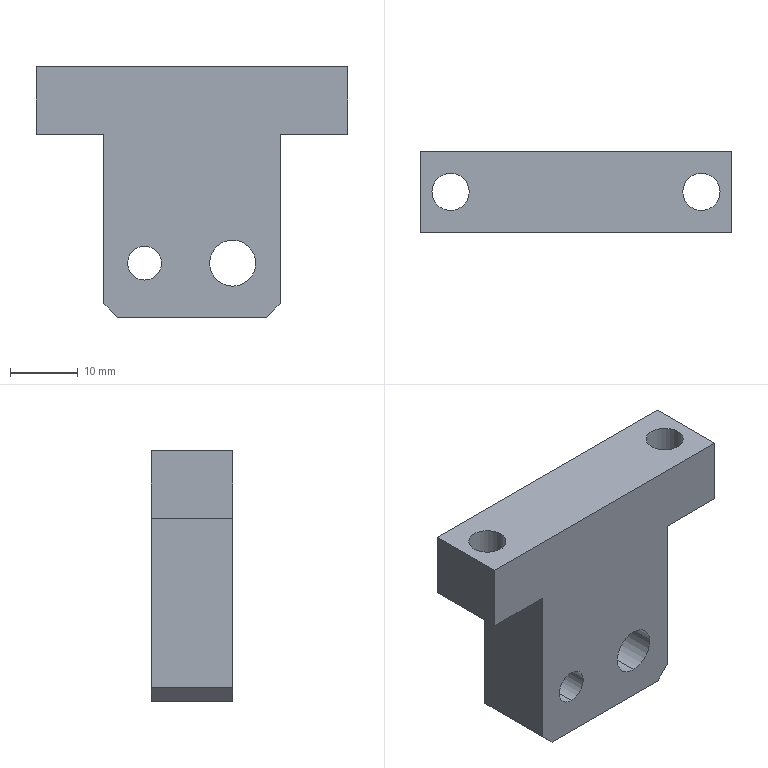Part | NX | features BREP 1 | 1 solid | 20 faces | box 46 x 12 x 37 mm | volume 12749 mm3 | plane 12 | cylinder 8 | commonest cylinder face diameters 5.5 x4 5 x2 6.8 x2
STEP:
#1=CARTESIAN_POINT('',(-20.051,-130.878,4.6));
#2=VERTEX_POINT('',#1);
#3=CARTESIAN_POINT('',(-20.051,-130.878,11.4));
#4=VERTEX_POINT('',#3);
#5=CARTESIAN_POINT('',(-20.051,-130.878,8.));
#6=DIRECTION('',(0.,1.,0.));
#7=DIRECTION('',(0.,0.,1.));
#8=AXIS2_PLACEMENT_3D('',#5,#6,#7);
#9=CIRCLE('',#8,3.4);
#10=EDGE_CURVE('',#2,#4,#9,.T.);
#11=ORIENTED_EDGE('',*,*,#10,.F.);
#12=CARTESIAN_POINT('',(-20.051,-118.878,4.6));
#13=VERTEX_POINT('',#12);
#14=CARTESIAN_POINT('',(-20.051,-118.878,4.6));
#15=DIRECTION('',(0.,1.,0.));
#16=VECTOR('',#15,1000.);
#17=LINE('',#14,#16);
#18=EDGE_CURVE('',#13,#2,#17,.F.);
#19=ORIENTED_EDGE('',*,*,#18,.F.);
#20=CARTESIAN_POINT('',(-20.051,-118.878,11.4));
#21=VERTEX_POINT('',#20);
#22=CARTESIAN_POINT('',(-20.051,-118.878,8.));
#23=DIRECTION('',(0.,1.,0.));
#24=DIRECTION('',(0.,0.,1.));
#25=AXIS2_PLACEMENT_3D('',#22,#23,#24);
#26=CIRCLE('',#25,3.4);
#27=EDGE_CURVE('',#13,#21,#26,.T.);
#28=ORIENTED_EDGE('',*,*,#27,.T.);
#29=CARTESIAN_POINT('',(-20.051,-118.878,11.4));
#30=DIRECTION('',(0.,1.,0.));
#31=VECTOR('',#30,1000.);
#32=LINE('',#29,#31);
#33=EDGE_CURVE('',#21,#4,#32,.F.);
#34=ORIENTED_EDGE('',*,*,#33,.T.);
#35=EDGE_LOOP('',(#11,#19,#28,#34));
#36=FACE_BOUND('',#35,.T.);
#37=CARTESIAN_POINT('',(-20.051,-118.878,8.));
#38=DIRECTION('',(0.,1.,0.));
#39=DIRECTION('',(0.,0.,1.));
#40=AXIS2_PLACEMENT_3D('',#37,#38,#39);
#41=CYLINDRICAL_SURFACE('',#40,3.4);
#42=ADVANCED_FACE('',(#36),#41,.F.);
#43=CARTESIAN_POINT('',(-41.801,-124.878,37.));
#44=VERTEX_POINT('',#43);
#45=CARTESIAN_POINT('',(-47.301,-124.878,37.));
#46=VERTEX_POINT('',#45);
#47=CARTESIAN_POINT('',(-44.551,-124.878,37.));
#48=DIRECTION('',(0.,0.,-1.));
#49=DIRECTION('',(-1.,0.,0.));
#50=AXIS2_PLACEMENT_3D('',#47,#48,#49);
#51=CIRCLE('',#50,2.75);
#52=EDGE_CURVE('',#44,#46,#51,.T.);
#53=ORIENTED_EDGE('',*,*,#52,.F.);
#54=CARTESIAN_POINT('',(-41.801,-124.878,27.));
#55=VERTEX_POINT('',#54);
#56=CARTESIAN_POINT('',(-41.801,-124.878,37.));
#57=DIRECTION('',(0.,0.,-1.));
#58=VECTOR('',#57,1000.);
#59=LINE('',#56,#58);
#60=EDGE_CURVE('',#44,#55,#59,.T.);
#61=ORIENTED_EDGE('',*,*,#60,.T.);
#62=CARTESIAN_POINT('',(-47.301,-124.878,27.));
#63=VERTEX_POINT('',#62);
#64=CARTESIAN_POINT('',(-44.551,-124.878,27.));
#65=DIRECTION('',(0.,0.,-1.));
#66=DIRECTION('',(-1.,0.,0.));
#67=AXIS2_PLACEMENT_3D('',#64,#65,#66);
#68=CIRCLE('',#67,2.75);
#69=EDGE_CURVE('',#55,#63,#68,.T.);
#70=ORIENTED_EDGE('',*,*,#69,.T.);
#71=CARTESIAN_POINT('',(-47.301,-124.878,37.));
#72=DIRECTION('',(0.,0.,-1.));
#73=VECTOR('',#72,1000.);
#74=LINE('',#71,#73);
#75=EDGE_CURVE('',#46,#63,#74,.T.);
#76=ORIENTED_EDGE('',*,*,#75,.F.);
#77=EDGE_LOOP('',(#53,#61,#70,#76));
#78=FACE_BOUND('',#77,.T.);
#79=CARTESIAN_POINT('',(-44.551,-124.878,37.));
#80=DIRECTION('',(0.,0.,-1.));
#81=DIRECTION('',(-1.,0.,0.));
#82=AXIS2_PLACEMENT_3D('',#79,#80,#81);
#83=CYLINDRICAL_SURFACE('',#82,2.75);
#84=ADVANCED_FACE('',(#78),#83,.F.);
#85=CARTESIAN_POINT('',(-4.801,-124.878,37.));
#86=VERTEX_POINT('',#85);
#87=CARTESIAN_POINT('',(-10.301,-124.878,37.));
#88=VERTEX_POINT('',#87);
#89=CARTESIAN_POINT('',(-7.551,-124.878,37.));
#90=DIRECTION('',(0.,0.,-1.));
#91=DIRECTION('',(-1.,0.,0.));
#92=AXIS2_PLACEMENT_3D('',#89,#90,#91);
#93=CIRCLE('',#92,2.75);
#94=EDGE_CURVE('',#86,#88,#93,.T.);
#95=ORIENTED_EDGE('',*,*,#94,.F.);
#96=CARTESIAN_POINT('',(-4.801,-124.878,27.));
#97=VERTEX_POINT('',#96);
#98=CARTESIAN_POINT('',(-4.801,-124.878,37.));
#99=DIRECTION('',(0.,0.,-1.));
#100=VECTOR('',#99,1000.);
#101=LINE('',#98,#100);
#102=EDGE_CURVE('',#86,#97,#101,.T.);
#103=ORIENTED_EDGE('',*,*,#102,.T.);
#104=CARTESIAN_POINT('',(-10.301,-124.878,27.));
#105=VERTEX_POINT('',#104);
#106=CARTESIAN_POINT('',(-7.551,-124.878,27.));
#107=DIRECTION('',(0.,0.,-1.));
#108=DIRECTION('',(-1.,0.,0.));
#109=AXIS2_PLACEMENT_3D('',#106,#107,#108);
#110=CIRCLE('',#109,2.75);
#111=EDGE_CURVE('',#97,#105,#110,.T.);
#112=ORIENTED_EDGE('',*,*,#111,.T.);
#113=CARTESIAN_POINT('',(-10.301,-124.878,37.));
#114=DIRECTION('',(0.,0.,-1.));
#115=VECTOR('',#114,1000.);
#116=LINE('',#113,#115);
#117=EDGE_CURVE('',#88,#105,#116,.T.);
#118=ORIENTED_EDGE('',*,*,#117,.F.);
#119=EDGE_LOOP('',(#95,#103,#112,#118));
#120=FACE_BOUND('',#119,.T.);
#121=CARTESIAN_POINT('',(-7.551,-124.878,37.));
#122=DIRECTION('',(0.,0.,-1.));
#123=DIRECTION('',(-1.,0.,0.));
#124=AXIS2_PLACEMENT_3D('',#121,#122,#123);
#125=CYLINDRICAL_SURFACE('',#124,2.75);
#126=ADVANCED_FACE('',(#120),#125,.F.);
#127=CARTESIAN_POINT('',(-33.051,-130.878,5.5));
#128=VERTEX_POINT('',#127);
#129=CARTESIAN_POINT('',(-33.051,-130.878,10.5));
#130=VERTEX_POINT('',#129);
#131=CARTESIAN_POINT('',(-33.051,-130.878,8.));
#132=DIRECTION('',(0.,1.,0.));
#133=DIRECTION('',(0.,0.,1.));
#134=AXIS2_PLACEMENT_3D('',#131,#132,#133);
#135=CIRCLE('',#134,2.5);
#136=EDGE_CURVE('',#128,#130,#135,.T.);
#137=ORIENTED_EDGE('',*,*,#136,.F.);
#138=CARTESIAN_POINT('',(-33.051,-118.878,5.5));
#139=VERTEX_POINT('',#138);
#140=CARTESIAN_POINT('',(-33.051,-118.878,5.5));
#141=DIRECTION('',(0.,1.,0.));
#142=VECTOR('',#141,1000.);
#143=LINE('',#140,#142);
#144=EDGE_CURVE('',#139,#128,#143,.F.);
#145=ORIENTED_EDGE('',*,*,#144,.F.);
#146=CARTESIAN_POINT('',(-33.051,-118.878,10.5));
#147=VERTEX_POINT('',#146);
#148=CARTESIAN_POINT('',(-33.051,-118.878,8.));
#149=DIRECTION('',(0.,1.,0.));
#150=DIRECTION('',(0.,0.,1.));
#151=AXIS2_PLACEMENT_3D('',#148,#149,#150);
#152=CIRCLE('',#151,2.5);
#153=EDGE_CURVE('',#139,#147,#152,.T.);
#154=ORIENTED_EDGE('',*,*,#153,.T.);
#155=CARTESIAN_POINT('',(-33.051,-118.878,10.5));
#156=DIRECTION('',(0.,1.,0.));
#157=VECTOR('',#156,1000.);
#158=LINE('',#155,#157);
#159=EDGE_CURVE('',#147,#130,#158,.F.);
#160=ORIENTED_EDGE('',*,*,#159,.T.);
#161=EDGE_LOOP('',(#137,#145,#154,#160));
#162=FACE_BOUND('',#161,.T.);
#163=CARTESIAN_POINT('',(-33.051,-118.878,8.));
#164=DIRECTION('',(0.,1.,0.));
#165=DIRECTION('',(0.,0.,1.));
#166=AXIS2_PLACEMENT_3D('',#163,#164,#165);
#167=CYLINDRICAL_SURFACE('',#166,2.5);
#168=ADVANCED_FACE('',(#162),#167,.F.);
#169=CARTESIAN_POINT('',(-13.051,-118.878,27.));
#170=VERTEX_POINT('',#169);
#171=CARTESIAN_POINT('',(-13.051,-118.878,2.));
#172=VERTEX_POINT('',#171);
#173=CARTESIAN_POINT('',(-13.051,-118.878,27.));
#174=DIRECTION('',(0.,0.,-1.));
#175=VECTOR('',#174,1000.);
#176=LINE('',#173,#175);
#177=EDGE_CURVE('',#170,#172,#176,.T.);
#178=ORIENTED_EDGE('',*,*,#177,.T.);
#179=CARTESIAN_POINT('',(-15.051,-118.878,0.));
#180=VERTEX_POINT('',#179);
#181=CARTESIAN_POINT('',(-13.051,-118.878,2.));
#182=DIRECTION('',(-0.7071,0.,-0.7071));
#183=VECTOR('',#182,1000.);
#184=LINE('',#181,#183);
#185=EDGE_CURVE('',#172,#180,#184,.T.);
#186=ORIENTED_EDGE('',*,*,#185,.T.);
#187=CARTESIAN_POINT('',(-37.051,-118.878,0.));
#188=VERTEX_POINT('',#187);
#189=CARTESIAN_POINT('',(-39.051,-118.878,0.));
#190=DIRECTION('',(-1.,0.,0.));
#191=VECTOR('',#190,1000.);
#192=LINE('',#189,#191);
#193=EDGE_CURVE('',#180,#188,#192,.T.);
#194=ORIENTED_EDGE('',*,*,#193,.T.);
#195=CARTESIAN_POINT('',(-39.051,-118.878,2.));
#196=VERTEX_POINT('',#195);
#197=CARTESIAN_POINT('',(-39.051,-118.878,2.));
#198=DIRECTION('',(-0.7071,0.,0.7071));
#199=VECTOR('',#198,1000.);
#200=LINE('',#197,#199);
#201=EDGE_CURVE('',#188,#196,#200,.T.);
#202=ORIENTED_EDGE('',*,*,#201,.T.);
#203=CARTESIAN_POINT('',(-39.051,-118.878,27.));
#204=VERTEX_POINT('',#203);
#205=CARTESIAN_POINT('',(-39.051,-118.878,27.));
#206=DIRECTION('',(0.,0.,-1.));
#207=VECTOR('',#206,1000.);
#208=LINE('',#205,#207);
#209=EDGE_CURVE('',#204,#196,#208,.T.);
#210=ORIENTED_EDGE('',*,*,#209,.F.);
#211=CARTESIAN_POINT('',(-49.051,-118.878,27.));
#212=VERTEX_POINT('',#211);
#213=CARTESIAN_POINT('',(-49.051,-118.878,27.));
#214=DIRECTION('',(-1.,0.,0.));
#215=VECTOR('',#214,1000.);
#216=LINE('',#213,#215);
#217=EDGE_CURVE('',#204,#212,#216,.T.);
#218=ORIENTED_EDGE('',*,*,#217,.T.);
#219=CARTESIAN_POINT('',(-49.051,-118.878,37.));
#220=VERTEX_POINT('',#219);
#221=CARTESIAN_POINT('',(-49.051,-118.878,37.));
#222=DIRECTION('',(0.,0.,-1.));
#223=VECTOR('',#222,1000.);
#224=LINE('',#221,#223);
#225=EDGE_CURVE('',#220,#212,#224,.T.);
#226=ORIENTED_EDGE('',*,*,#225,.F.);
#227=CARTESIAN_POINT('',(-3.051,-118.878,37.));
#228=VERTEX_POINT('',#227);
#229=CARTESIAN_POINT('',(-49.051,-118.878,37.));
#230=DIRECTION('',(-1.,0.,0.));
#231=VECTOR('',#230,1000.);
#232=LINE('',#229,#231);
#233=EDGE_CURVE('',#228,#220,#232,.T.);
#234=ORIENTED_EDGE('',*,*,#233,.F.);
#235=CARTESIAN_POINT('',(-3.051,-118.878,27.));
#236=VERTEX_POINT('',#235);
#237=CARTESIAN_POINT('',(-3.051,-118.878,37.));
#238=DIRECTION('',(0.,0.,-1.));
#239=VECTOR('',#238,1000.);
#240=LINE('',#237,#239);
#241=EDGE_CURVE('',#228,#236,#240,.T.);
#242=ORIENTED_EDGE('',*,*,#241,.T.);
#243=CARTESIAN_POINT('',(-49.051,-118.878,27.));
#244=DIRECTION('',(-1.,0.,0.));
#245=VECTOR('',#244,1000.);
#246=LINE('',#243,#245);
#247=EDGE_CURVE('',#236,#170,#246,.T.);
#248=ORIENTED_EDGE('',*,*,#247,.T.);
#249=EDGE_LOOP('',(#178,#186,#194,#202,#210,#218,#226,#234,#242,#248));
#250=FACE_BOUND('',#249,.T.);
#251=CARTESIAN_POINT('',(-33.051,-118.878,8.));
#252=DIRECTION('',(0.,1.,0.));
#253=DIRECTION('',(0.,0.,1.));
#254=AXIS2_PLACEMENT_3D('',#251,#252,#253);
#255=CIRCLE('',#254,2.5);
#256=EDGE_CURVE('',#147,#139,#255,.T.);
#257=ORIENTED_EDGE('',*,*,#256,.F.);
#258=ORIENTED_EDGE('',*,*,#153,.F.);
#259=EDGE_LOOP('',(#257,#258));
#260=FACE_BOUND('',#259,.T.);
#261=CARTESIAN_POINT('',(-20.051,-118.878,8.));
#262=DIRECTION('',(0.,1.,0.));
#263=DIRECTION('',(0.,0.,1.));
#264=AXIS2_PLACEMENT_3D('',#261,#262,#263);
#265=CIRCLE('',#264,3.4);
#266=EDGE_CURVE('',#21,#13,#265,.T.);
#267=ORIENTED_EDGE('',*,*,#266,.F.);
#268=ORIENTED_EDGE('',*,*,#27,.F.);
#269=EDGE_LOOP('',(#267,#268));
#270=FACE_BOUND('',#269,.T.);
#271=CARTESIAN_POINT('',(-39.051,-118.878,27.));
#272=DIRECTION('',(0.,-1.,0.));
#273=DIRECTION('',(0.,0.,-1.));
#274=AXIS2_PLACEMENT_3D('',#271,#272,#273);
#275=PLANE('',#274);
#276=ADVANCED_FACE('',(#250,#260,#270),#275,.F.);
#277=ORIENTED_EDGE('',*,*,#209,.T.);
#278=CARTESIAN_POINT('',(-39.051,-130.878,2.));
#279=VERTEX_POINT('',#278);
#280=CARTESIAN_POINT('',(-39.051,-130.878,2.));
#281=DIRECTION('',(0.,-1.,0.));
#282=VECTOR('',#281,1000.);
#283=LINE('',#280,#282);
#284=EDGE_CURVE('',#196,#279,#283,.T.);
#285=ORIENTED_EDGE('',*,*,#284,.T.);
#286=CARTESIAN_POINT('',(-39.051,-130.878,27.));
#287=VERTEX_POINT('',#286);
#288=CARTESIAN_POINT('',(-39.051,-130.878,27.));
#289=DIRECTION('',(0.,0.,-1.));
#290=VECTOR('',#289,1000.);
#291=LINE('',#288,#290);
#292=EDGE_CURVE('',#287,#279,#291,.T.);
#293=ORIENTED_EDGE('',*,*,#292,.F.);
#294=CARTESIAN_POINT('',(-39.051,-130.878,27.));
#295=DIRECTION('',(0.,-1.,0.));
#296=VECTOR('',#295,1000.);
#297=LINE('',#294,#296);
#298=EDGE_CURVE('',#204,#287,#297,.T.);
#299=ORIENTED_EDGE('',*,*,#298,.F.);
#300=EDGE_LOOP('',(#277,#285,#293,#299));
#301=FACE_BOUND('',#300,.T.);
#302=CARTESIAN_POINT('',(-39.051,-130.878,27.));
#303=DIRECTION('',(1.,0.,0.));
#304=DIRECTION('',(0.,1.,0.));
#305=AXIS2_PLACEMENT_3D('',#302,#303,#304);
#306=PLANE('',#305);
#307=ADVANCED_FACE('',(#301),#306,.F.);
#308=CARTESIAN_POINT('',(-37.051,-130.878,0.));
#309=VERTEX_POINT('',#308);
#310=CARTESIAN_POINT('',(-15.051,-130.878,0.));
#311=VERTEX_POINT('',#310);
#312=CARTESIAN_POINT('',(-39.051,-130.878,0.));
#313=DIRECTION('',(1.,0.,0.));
#314=VECTOR('',#313,1000.);
#315=LINE('',#312,#314);
#316=EDGE_CURVE('',#309,#311,#315,.T.);
#317=ORIENTED_EDGE('',*,*,#316,.T.);
#318=CARTESIAN_POINT('',(-13.051,-130.878,2.));
#319=VERTEX_POINT('',#318);
#320=CARTESIAN_POINT('',(-13.051,-130.878,2.));
#321=DIRECTION('',(0.7071,0.,0.7071));
#322=VECTOR('',#321,1000.);
#323=LINE('',#320,#322);
#324=EDGE_CURVE('',#311,#319,#323,.T.);
#325=ORIENTED_EDGE('',*,*,#324,.T.);
#326=CARTESIAN_POINT('',(-13.051,-130.878,27.));
#327=VERTEX_POINT('',#326);
#328=CARTESIAN_POINT('',(-13.051,-130.878,27.));
#329=DIRECTION('',(0.,0.,-1.));
#330=VECTOR('',#329,1000.);
#331=LINE('',#328,#330);
#332=EDGE_CURVE('',#327,#319,#331,.T.);
#333=ORIENTED_EDGE('',*,*,#332,.F.);
#334=CARTESIAN_POINT('',(-3.051,-130.878,27.));
#335=VERTEX_POINT('',#334);
#336=CARTESIAN_POINT('',(-49.051,-130.878,27.));
#337=DIRECTION('',(1.,0.,0.));
#338=VECTOR('',#337,1000.);
#339=LINE('',#336,#338);
#340=EDGE_CURVE('',#327,#335,#339,.T.);
#341=ORIENTED_EDGE('',*,*,#340,.T.);
#342=CARTESIAN_POINT('',(-3.051,-130.878,37.));
#343=VERTEX_POINT('',#342);
#344=CARTESIAN_POINT('',(-3.051,-130.878,37.));
#345=DIRECTION('',(0.,0.,-1.));
#346=VECTOR('',#345,1000.);
#347=LINE('',#344,#346);
#348=EDGE_CURVE('',#343,#335,#347,.T.);
#349=ORIENTED_EDGE('',*,*,#348,.F.);
#350=CARTESIAN_POINT('',(-49.051,-130.878,37.));
#351=VERTEX_POINT('',#350);
#352=CARTESIAN_POINT('',(-49.051,-130.878,37.));
#353=DIRECTION('',(1.,0.,0.));
#354=VECTOR('',#353,1000.);
#355=LINE('',#352,#354);
#356=EDGE_CURVE('',#351,#343,#355,.T.);
#357=ORIENTED_EDGE('',*,*,#356,.F.);
#358=CARTESIAN_POINT('',(-49.051,-130.878,27.));
#359=VERTEX_POINT('',#358);
#360=CARTESIAN_POINT('',(-49.051,-130.878,37.));
#361=DIRECTION('',(0.,0.,-1.));
#362=VECTOR('',#361,1000.);
#363=LINE('',#360,#362);
#364=EDGE_CURVE('',#351,#359,#363,.T.);
#365=ORIENTED_EDGE('',*,*,#364,.T.);
#366=CARTESIAN_POINT('',(-49.051,-130.878,27.));
#367=DIRECTION('',(1.,0.,0.));
#368=VECTOR('',#367,1000.);
#369=LINE('',#366,#368);
#370=EDGE_CURVE('',#359,#287,#369,.T.);
#371=ORIENTED_EDGE('',*,*,#370,.T.);
#372=ORIENTED_EDGE('',*,*,#292,.T.);
#373=CARTESIAN_POINT('',(-39.051,-130.878,2.));
#374=DIRECTION('',(0.7071,0.,-0.7071));
#375=VECTOR('',#374,1000.);
#376=LINE('',#373,#375);
#377=EDGE_CURVE('',#279,#309,#376,.T.);
#378=ORIENTED_EDGE('',*,*,#377,.T.);
#379=EDGE_LOOP('',(#317,#325,#333,#341,#349,#357,#365,#371,#372,#378));
#380=FACE_BOUND('',#379,.T.);
#381=CARTESIAN_POINT('',(-20.051,-130.878,8.));
#382=DIRECTION('',(0.,1.,0.));
#383=DIRECTION('',(0.,0.,1.));
#384=AXIS2_PLACEMENT_3D('',#381,#382,#383);
#385=CIRCLE('',#384,3.4);
#386=EDGE_CURVE('',#4,#2,#385,.T.);
#387=ORIENTED_EDGE('',*,*,#386,.T.);
#388=ORIENTED_EDGE('',*,*,#10,.T.);
#389=EDGE_LOOP('',(#387,#388));
#390=FACE_BOUND('',#389,.T.);
#391=CARTESIAN_POINT('',(-33.051,-130.878,8.));
#392=DIRECTION('',(0.,1.,0.));
#393=DIRECTION('',(0.,0.,1.));
#394=AXIS2_PLACEMENT_3D('',#391,#392,#393);
#395=CIRCLE('',#394,2.5);
#396=EDGE_CURVE('',#130,#128,#395,.T.);
#397=ORIENTED_EDGE('',*,*,#396,.T.);
#398=ORIENTED_EDGE('',*,*,#136,.T.);
#399=EDGE_LOOP('',(#397,#398));
#400=FACE_BOUND('',#399,.T.);
#401=CARTESIAN_POINT('',(-39.051,-130.878,27.));
#402=DIRECTION('',(0.,1.,0.));
#403=DIRECTION('',(1.,0.,0.));
#404=AXIS2_PLACEMENT_3D('',#401,#402,#403);
#405=PLANE('',#404);
#406=ADVANCED_FACE('',(#380,#390,#400),#405,.F.);
#407=ORIENTED_EDGE('',*,*,#332,.T.);
#408=CARTESIAN_POINT('',(-13.051,-118.878,2.));
#409=DIRECTION('',(0.,1.,0.));
#410=VECTOR('',#409,1000.);
#411=LINE('',#408,#410);
#412=EDGE_CURVE('',#319,#172,#411,.T.);
#413=ORIENTED_EDGE('',*,*,#412,.T.);
#414=ORIENTED_EDGE('',*,*,#177,.F.);
#415=CARTESIAN_POINT('',(-13.051,-130.878,27.));
#416=DIRECTION('',(0.,1.,0.));
#417=VECTOR('',#416,1000.);
#418=LINE('',#415,#417);
#419=EDGE_CURVE('',#327,#170,#418,.T.);
#420=ORIENTED_EDGE('',*,*,#419,.F.);
#421=EDGE_LOOP('',(#407,#413,#414,#420));
#422=FACE_BOUND('',#421,.T.);
#423=CARTESIAN_POINT('',(-13.051,-130.878,27.));
#424=DIRECTION('',(-1.,0.,0.));
#425=DIRECTION('',(0.,0.,1.));
#426=AXIS2_PLACEMENT_3D('',#423,#424,#425);
#427=PLANE('',#426);
#428=ADVANCED_FACE('',(#422),#427,.F.);
#429=ORIENTED_EDGE('',*,*,#193,.F.);
#430=CARTESIAN_POINT('',(-15.051,-130.878,0.));
#431=DIRECTION('',(0.,-1.,0.));
#432=VECTOR('',#431,1000.);
#433=LINE('',#430,#432);
#434=EDGE_CURVE('',#180,#311,#433,.T.);
#435=ORIENTED_EDGE('',*,*,#434,.T.);
#436=ORIENTED_EDGE('',*,*,#316,.F.);
#437=CARTESIAN_POINT('',(-37.051,-118.878,0.));
#438=DIRECTION('',(0.,1.,0.));
#439=VECTOR('',#438,1000.);
#440=LINE('',#437,#439);
#441=EDGE_CURVE('',#309,#188,#440,.T.);
#442=ORIENTED_EDGE('',*,*,#441,.T.);
#443=EDGE_LOOP('',(#429,#435,#436,#442));
#444=FACE_BOUND('',#443,.T.);
#445=CARTESIAN_POINT('',(-39.051,-118.878,0.));
#446=DIRECTION('',(0.,0.,-1.));
#447=DIRECTION('',(0.,-1.,0.));
#448=AXIS2_PLACEMENT_3D('',#445,#446,#447);
#449=PLANE('',#448);
#450=ADVANCED_FACE('',(#444),#449,.T.);
#451=ORIENTED_EDGE('',*,*,#217,.F.);
#452=ORIENTED_EDGE('',*,*,#298,.T.);
#453=ORIENTED_EDGE('',*,*,#370,.F.);
#454=CARTESIAN_POINT('',(-49.051,-118.878,27.));
#455=DIRECTION('',(0.,-1.,0.));
#456=VECTOR('',#455,1000.);
#457=LINE('',#454,#456);
#458=EDGE_CURVE('',#212,#359,#457,.T.);
#459=ORIENTED_EDGE('',*,*,#458,.F.);
#460=EDGE_LOOP('',(#451,#452,#453,#459));
#461=FACE_BOUND('',#460,.T.);
#462=CARTESIAN_POINT('',(-44.551,-124.878,27.));
#463=DIRECTION('',(0.,0.,-1.));
#464=DIRECTION('',(-1.,0.,0.));
#465=AXIS2_PLACEMENT_3D('',#462,#463,#464);
#466=CIRCLE('',#465,2.75);
#467=EDGE_CURVE('',#63,#55,#466,.T.);
#468=ORIENTED_EDGE('',*,*,#467,.F.);
#469=ORIENTED_EDGE('',*,*,#69,.F.);
#470=EDGE_LOOP('',(#468,#469));
#471=FACE_BOUND('',#470,.T.);
#472=CARTESIAN_POINT('',(-49.051,-130.878,27.));
#473=DIRECTION('',(0.,0.,1.));
#474=DIRECTION('',(1.,0.,0.));
#475=AXIS2_PLACEMENT_3D('',#472,#473,#474);
#476=PLANE('',#475);
#477=ADVANCED_FACE('',(#461,#471),#476,.F.);
#478=ORIENTED_EDGE('',*,*,#340,.F.);
#479=ORIENTED_EDGE('',*,*,#419,.T.);
#480=ORIENTED_EDGE('',*,*,#247,.F.);
#481=CARTESIAN_POINT('',(-3.051,-118.878,27.));
#482=DIRECTION('',(0.,1.,0.));
#483=VECTOR('',#482,1000.);
#484=LINE('',#481,#483);
#485=EDGE_CURVE('',#335,#236,#484,.T.);
#486=ORIENTED_EDGE('',*,*,#485,.F.);
#487=EDGE_LOOP('',(#478,#479,#480,#486));
#488=FACE_BOUND('',#487,.T.);
#489=CARTESIAN_POINT('',(-7.551,-124.878,27.));
#490=DIRECTION('',(0.,0.,-1.));
#491=DIRECTION('',(-1.,0.,0.));
#492=AXIS2_PLACEMENT_3D('',#489,#490,#491);
#493=CIRCLE('',#492,2.75);
#494=EDGE_CURVE('',#105,#97,#493,.T.);
#495=ORIENTED_EDGE('',*,*,#494,.F.);
#496=ORIENTED_EDGE('',*,*,#111,.F.);
#497=EDGE_LOOP('',(#495,#496));
#498=FACE_BOUND('',#497,.T.);
#499=CARTESIAN_POINT('',(-49.051,-130.878,27.));
#500=DIRECTION('',(0.,0.,1.));
#501=DIRECTION('',(1.,0.,0.));
#502=AXIS2_PLACEMENT_3D('',#499,#500,#501);
#503=PLANE('',#502);
#504=ADVANCED_FACE('',(#488,#498),#503,.F.);
#505=ORIENTED_EDGE('',*,*,#458,.T.);
#506=ORIENTED_EDGE('',*,*,#364,.F.);
#507=CARTESIAN_POINT('',(-49.051,-118.878,37.));
#508=DIRECTION('',(0.,-1.,0.));
#509=VECTOR('',#508,1000.);
#510=LINE('',#507,#509);
#511=EDGE_CURVE('',#220,#351,#510,.T.);
#512=ORIENTED_EDGE('',*,*,#511,.F.);
#513=ORIENTED_EDGE('',*,*,#225,.T.);
#514=EDGE_LOOP('',(#505,#506,#512,#513));
#515=FACE_BOUND('',#514,.T.);
#516=CARTESIAN_POINT('',(-49.051,-118.878,37.));
#517=DIRECTION('',(1.,0.,0.));
#518=DIRECTION('',(0.,1.,0.));
#519=AXIS2_PLACEMENT_3D('',#516,#517,#518);
#520=PLANE('',#519);
#521=ADVANCED_FACE('',(#515),#520,.F.);
#522=ORIENTED_EDGE('',*,*,#485,.T.);
#523=ORIENTED_EDGE('',*,*,#241,.F.);
#524=CARTESIAN_POINT('',(-3.051,-118.878,37.));
#525=DIRECTION('',(0.,1.,0.));
#526=VECTOR('',#525,1000.);
#527=LINE('',#524,#526);
#528=EDGE_CURVE('',#343,#228,#527,.T.);
#529=ORIENTED_EDGE('',*,*,#528,.F.);
#530=ORIENTED_EDGE('',*,*,#348,.T.);
#531=EDGE_LOOP('',(#522,#523,#529,#530));
#532=FACE_BOUND('',#531,.T.);
#533=CARTESIAN_POINT('',(-3.051,-118.878,37.));
#534=DIRECTION('',(-1.,0.,0.));
#535=DIRECTION('',(0.,0.,1.));
#536=AXIS2_PLACEMENT_3D('',#533,#534,#535);
#537=PLANE('',#536);
#538=ADVANCED_FACE('',(#532),#537,.F.);
#539=ORIENTED_EDGE('',*,*,#511,.T.);
#540=ORIENTED_EDGE('',*,*,#356,.T.);
#541=ORIENTED_EDGE('',*,*,#528,.T.);
#542=ORIENTED_EDGE('',*,*,#233,.T.);
#543=EDGE_LOOP('',(#539,#540,#541,#542));
#544=FACE_BOUND('',#543,.T.);
#545=CARTESIAN_POINT('',(-44.551,-124.878,37.));
#546=DIRECTION('',(0.,0.,-1.));
#547=DIRECTION('',(-1.,0.,0.));
#548=AXIS2_PLACEMENT_3D('',#545,#546,#547);
#549=CIRCLE('',#548,2.75);
#550=EDGE_CURVE('',#46,#44,#549,.T.);
#551=ORIENTED_EDGE('',*,*,#550,.T.);
#552=ORIENTED_EDGE('',*,*,#52,.T.);
#553=EDGE_LOOP('',(#551,#552));
#554=FACE_BOUND('',#553,.T.);
#555=CARTESIAN_POINT('',(-7.551,-124.878,37.));
#556=DIRECTION('',(0.,0.,-1.));
#557=DIRECTION('',(-1.,0.,0.));
#558=AXIS2_PLACEMENT_3D('',#555,#556,#557);
#559=CIRCLE('',#558,2.75);
#560=EDGE_CURVE('',#88,#86,#559,.T.);
#561=ORIENTED_EDGE('',*,*,#560,.T.);
#562=ORIENTED_EDGE('',*,*,#94,.T.);
#563=EDGE_LOOP('',(#561,#562));
#564=FACE_BOUND('',#563,.T.);
#565=CARTESIAN_POINT('',(-49.051,-130.878,37.));
#566=DIRECTION('',(0.,0.,1.));
#567=DIRECTION('',(1.,0.,0.));
#568=AXIS2_PLACEMENT_3D('',#565,#566,#567);
#569=PLANE('',#568);
#570=ADVANCED_FACE('',(#544,#554,#564),#569,.T.);
#571=ORIENTED_EDGE('',*,*,#144,.T.);
#572=ORIENTED_EDGE('',*,*,#396,.F.);
#573=ORIENTED_EDGE('',*,*,#159,.F.);
#574=ORIENTED_EDGE('',*,*,#256,.T.);
#575=EDGE_LOOP('',(#571,#572,#573,#574));
#576=FACE_BOUND('',#575,.T.);
#577=CARTESIAN_POINT('',(-33.051,-118.878,8.));
#578=DIRECTION('',(0.,1.,0.));
#579=DIRECTION('',(0.,0.,1.));
#580=AXIS2_PLACEMENT_3D('',#577,#578,#579);
#581=CYLINDRICAL_SURFACE('',#580,2.5);
#582=ADVANCED_FACE('',(#576),#581,.F.);
#583=ORIENTED_EDGE('',*,*,#102,.F.);
#584=ORIENTED_EDGE('',*,*,#560,.F.);
#585=ORIENTED_EDGE('',*,*,#117,.T.);
#586=ORIENTED_EDGE('',*,*,#494,.T.);
#587=EDGE_LOOP('',(#583,#584,#585,#586));
#588=FACE_BOUND('',#587,.T.);
#589=CARTESIAN_POINT('',(-7.551,-124.878,37.));
#590=DIRECTION('',(0.,0.,-1.));
#591=DIRECTION('',(-1.,0.,0.));
#592=AXIS2_PLACEMENT_3D('',#589,#590,#591);
#593=CYLINDRICAL_SURFACE('',#592,2.75);
#594=ADVANCED_FACE('',(#588),#593,.F.);
#595=ORIENTED_EDGE('',*,*,#60,.F.);
#596=ORIENTED_EDGE('',*,*,#550,.F.);
#597=ORIENTED_EDGE('',*,*,#75,.T.);
#598=ORIENTED_EDGE('',*,*,#467,.T.);
#599=EDGE_LOOP('',(#595,#596,#597,#598));
#600=FACE_BOUND('',#599,.T.);
#601=CARTESIAN_POINT('',(-44.551,-124.878,37.));
#602=DIRECTION('',(0.,0.,-1.));
#603=DIRECTION('',(-1.,0.,0.));
#604=AXIS2_PLACEMENT_3D('',#601,#602,#603);
#605=CYLINDRICAL_SURFACE('',#604,2.75);
#606=ADVANCED_FACE('',(#600),#605,.F.);
#607=ORIENTED_EDGE('',*,*,#18,.T.);
#608=ORIENTED_EDGE('',*,*,#386,.F.);
#609=ORIENTED_EDGE('',*,*,#33,.F.);
#610=ORIENTED_EDGE('',*,*,#266,.T.);
#611=EDGE_LOOP('',(#607,#608,#609,#610));
#612=FACE_BOUND('',#611,.T.);
#613=CARTESIAN_POINT('',(-20.051,-118.878,8.));
#614=DIRECTION('',(0.,1.,0.));
#615=DIRECTION('',(0.,0.,1.));
#616=AXIS2_PLACEMENT_3D('',#613,#614,#615);
#617=CYLINDRICAL_SURFACE('',#616,3.4);
#618=ADVANCED_FACE('',(#612),#617,.F.);
#619=ORIENTED_EDGE('',*,*,#324,.F.);
#620=ORIENTED_EDGE('',*,*,#434,.F.);
#621=ORIENTED_EDGE('',*,*,#185,.F.);
#622=ORIENTED_EDGE('',*,*,#412,.F.);
#623=EDGE_LOOP('',(#619,#620,#621,#622));
#624=FACE_BOUND('',#623,.T.);
#625=CARTESIAN_POINT('',(-13.051,-130.878,2.));
#626=DIRECTION('',(0.7071,0.,-0.7071));
#627=DIRECTION('',(0.,-1.,0.));
#628=AXIS2_PLACEMENT_3D('',#625,#626,#627);
#629=PLANE('',#628);
#630=ADVANCED_FACE('',(#624),#629,.T.);
#631=ORIENTED_EDGE('',*,*,#201,.F.);
#632=ORIENTED_EDGE('',*,*,#441,.F.);
#633=ORIENTED_EDGE('',*,*,#377,.F.);
#634=ORIENTED_EDGE('',*,*,#284,.F.);
#635=EDGE_LOOP('',(#631,#632,#633,#634));
#636=FACE_BOUND('',#635,.T.);
#637=CARTESIAN_POINT('',(-39.051,-130.878,2.));
#638=DIRECTION('',(-0.7071,0.,-0.7071));
#639=DIRECTION('',(-0.7071,0.,0.7071));
#640=AXIS2_PLACEMENT_3D('',#637,#638,#639);
#641=PLANE('',#640);
#642=ADVANCED_FACE('',(#636),#641,.T.);
#643=CLOSED_SHELL('',(#42,#84,#126,#168,#276,#307,#406,#428,#450,#477,#504,#521,#538,#570,#582,#594,#606,#618,#630,#642));
#644=MANIFOLD_SOLID_BREP('',#643);
#645=(LENGTH_UNIT()NAMED_UNIT(*)SI_UNIT(.MILLI.,.METRE.));
#646=UNCERTAINTY_MEASURE_WITH_UNIT(LENGTH_MEASURE(0.00001),#645,'','');
#647=(NAMED_UNIT(*)PLANE_ANGLE_UNIT()SI_UNIT($,.RADIAN.));
#648=(NAMED_UNIT(*)SI_UNIT($,.STERADIAN.)SOLID_ANGLE_UNIT());
#649=(GEOMETRIC_REPRESENTATION_CONTEXT(3)GLOBAL_UNCERTAINTY_ASSIGNED_CONTEXT((#646))GLOBAL_UNIT_ASSIGNED_CONTEXT((#645,#647,#648))REPRESENTATION_CONTEXT('',''));
#650=ADVANCED_BREP_SHAPE_REPRESENTATION('',(#644),#649);